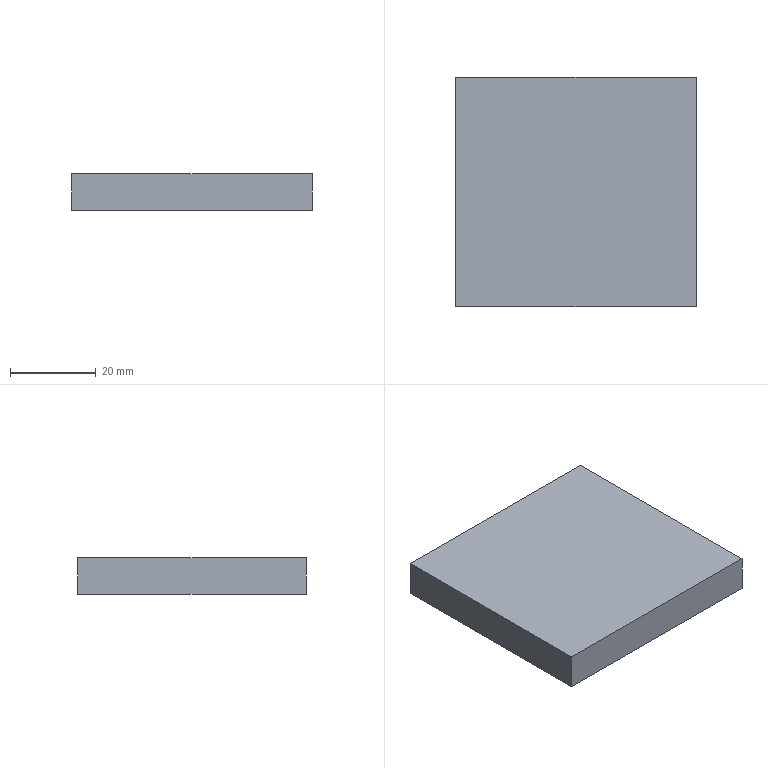NC program | NX | posted with a generic post | part box 56 x 53.3 x 8.5 mm
Lines 3580 to 5023 of 5023, first 1358 of 1432 lines:
(ZLEVEL_PROFILE_COPY_COPY , TOOL : D2)
N7134 T18 M6
N7136 G54
N7138 G17 G0 G90 X-10.995 Y-10.6 S9500 M3
N7140 G43 Z30. H18
N7142 Z-1.643
N7144 G94 G1 X-10.822 Y-10.9 F1000.
N7146 G3 X-10.648 Y-11. R0.2
N7148 G1 X-10. F1100.
N7150 G3 X-9.5 Y-10.5 R0.5
N7152 G1 Y-9.852
N7154 G3 X-9.6 Y-9.678 R0.2
N7156 G1 X-9.9 Y-9.505
N7158 G0 X-10.995 Y-10.6 Z-1.786
N7160 G1 X-10.822 Y-10.9 F1000.
N7162 G3 X-10.648 Y-11. R0.2
N7164 G1 X-10. F1100.
N7166 G3 X-9.5 Y-10.5 R0.5
N7168 G1 Y-9.852
N7170 G3 X-9.6 Y-9.678 R0.2
N7172 G1 X-9.9 Y-9.505
N7174 G0 X-10.995 Y-10.6 Z-1.929
N7176 G1 X-10.822 Y-10.9 F1000.
N7178 G3 X-10.648 Y-11. R0.2
N7180 G1 X-10. F1100.
N7182 G3 X-9.5 Y-10.5 R0.5
N7184 G1 Y-9.852
N7186 G3 X-9.6 Y-9.678 R0.2
N7188 G1 X-9.9 Y-9.505
N7190 G0 X-10.995 Y-10.6 Z-2.071
N7192 G1 X-10.822 Y-10.9 F1000.
N7194 G3 X-10.648 Y-11. R0.2
N7196 G1 X-10. F1100.
N7198 G3 X-9.5 Y-10.5 R0.5
N7200 G1 Y-9.852
N7202 G3 X-9.6 Y-9.678 R0.2
N7204 G1 X-9.9 Y-9.505
N7206 G0 X-10.995 Y-10.6 Z-2.214
N7208 G1 X-10.822 Y-10.9 F1000.
N7210 G3 X-10.648 Y-11. R0.2
N7212 G1 X-10. F1100.
N7214 G3 X-9.5 Y-10.5 R0.5
N7216 G1 Y-9.852
N7218 G3 X-9.6 Y-9.678 R0.2
N7220 G1 X-9.9 Y-9.505
N7222 G0 X-10.995 Y-10.6 Z-2.357
N7224 G1 X-10.822 Y-10.9 F1000.
N7226 G3 X-10.648 Y-11. R0.2
N7228 G1 X-10. F1100.
N7230 G3 X-9.5 Y-10.5 R0.5
N7232 G1 Y-9.852
N7234 G3 X-9.6 Y-9.678 R0.2
N7236 G1 X-9.9 Y-9.505
N7238 G0 X-10.995 Y-10.6 Z-2.5
N7240 G1 X-10.822 Y-10.9 F1000.
N7242 G3 X-10.648 Y-11. R0.2
N7244 G1 X-10. F1100.
N7246 G3 X-9.5 Y-10.5 R0.5
N7248 G1 Y-9.852
N7250 G3 X-9.6 Y-9.678 R0.2
N7252 G1 X-9.9 Y-9.505
N7254 G0 Z30.
N7256 X9.9
N7258 Z-1.643
N7260 G1 X9.6 Y-9.678 F1000.
N7262 G3 X9.5 Y-9.852 R0.2
N7264 G1 Y-10.5 F1100.
N7266 G3 X10. Y-11. R0.5
N7268 G1 X10.648
N7270 G3 X10.822 Y-10.9 R0.2
N7272 G1 X10.995 Y-10.6
N7274 G0 X9.9 Y-9.505 Z-1.786
N7276 G1 X9.6 Y-9.678 F1000.
N7278 G3 X9.5 Y-9.852 R0.2
N7280 G1 Y-10.5 F1100.
N7282 G3 X10. Y-11. R0.5
N7284 G1 X10.648
N7286 G3 X10.822 Y-10.9 R0.2
N7288 G1 X10.995 Y-10.6
N7290 G0 X9.9 Y-9.505 Z-1.929
N7292 G1 X9.6 Y-9.678 F1000.
N7294 G3 X9.5 Y-9.852 R0.2
N7296 G1 Y-10.5 F1100.
N7298 G3 X10. Y-11. R0.5
N7300 G1 X10.648
N7302 G3 X10.822 Y-10.9 R0.2
N7304 G1 X10.995 Y-10.6
N7306 G0 X9.9 Y-9.505 Z-2.071
N7308 G1 X9.6 Y-9.678 F1000.
N7310 G3 X9.5 Y-9.852 R0.2
N7312 G1 Y-10.5 F1100.
N7314 G3 X10. Y-11. R0.5
N7316 G1 X10.648
N7318 G3 X10.822 Y-10.9 R0.2
N7320 G1 X10.995 Y-10.6
N7322 G0 X9.9 Y-9.505 Z-2.214
N7324 G1 X9.6 Y-9.678 F1000.
N7326 G3 X9.5 Y-9.852 R0.2
N7328 G1 Y-10.5 F1100.
N7330 G3 X10. Y-11. R0.5
N7332 G1 X10.648
N7334 G3 X10.822 Y-10.9 R0.2
N7336 G1 X10.995 Y-10.6
N7338 G0 X9.9 Y-9.505 Z-2.357
N7340 G1 X9.6 Y-9.678 F1000.
N7342 G3 X9.5 Y-9.852 R0.2
N7344 G1 Y-10.5 F1100.
N7346 G3 X10. Y-11. R0.5
N7348 G1 X10.648
N7350 G3 X10.822 Y-10.9 R0.2
N7352 G1 X10.995 Y-10.6
N7354 G0 X9.9 Y-9.505 Z-2.5
N7356 G1 X9.6 Y-9.678 F1000.
N7358 G3 X9.5 Y-9.852 R0.2
N7360 G1 Y-10.5 F1100.
N7362 G3 X10. Y-11. R0.5
N7364 G1 X10.648
N7366 G3 X10.822 Y-10.9 R0.2
N7368 G1 X10.995 Y-10.6
N7370 G0 Z30.
N7372 X-20.908 Y-9.703
N7374 Z-1.643
N7376 G1 X-20.707 Y-9.425 F1000.
N7378 G3 X-20.686 Y-9.226 R0.2
N7380 G2 X-20.995 Y-8.5 R22.65 F1100.
N7382 G1 X-21.383
N7384 G2 X-21.769 Y-8.45 R1.5
N7386 G3 X-21.962 Y-8.502 R0.2
N7388 G1 X-22.183 Y-8.724
N7390 G0 X-20.908 Y-9.703 Z-1.786
N7392 G1 X-20.707 Y-9.425 F1000.
N7394 G3 X-20.686 Y-9.226 R0.2
N7396 G2 X-20.995 Y-8.5 R22.65 F1100.
N7398 G1 X-21.383
N7400 G2 X-21.769 Y-8.45 R1.5
N7402 G3 X-21.962 Y-8.502 R0.2
N7404 G1 X-22.183 Y-8.724
N7406 G0 X-20.908 Y-9.703 Z-1.929
N7408 G1 X-20.707 Y-9.425 F1000.
N7410 G3 X-20.686 Y-9.226 R0.2
N7412 G2 X-20.995 Y-8.5 R22.65 F1100.
N7414 G1 X-21.383
N7416 G2 X-21.769 Y-8.45 R1.5
N7418 G3 X-21.962 Y-8.502 R0.2
N7420 G1 X-22.183 Y-8.724
N7422 G0 X-20.908 Y-9.703 Z-2.071
N7424 G1 X-20.707 Y-9.425 F1000.
N7426 G3 X-20.686 Y-9.226 R0.2
N7428 G2 X-20.995 Y-8.5 R22.65 F1100.
N7430 G1 X-21.383
N7432 G2 X-21.769 Y-8.45 R1.5
N7434 G3 X-21.962 Y-8.502 R0.2
N7436 G1 X-22.183 Y-8.724
N7438 G0 X-20.908 Y-9.703 Z-2.214
N7440 G1 X-20.707 Y-9.425 F1000.
N7442 G3 X-20.686 Y-9.226 R0.2
N7444 G2 X-20.995 Y-8.5 R22.65 F1100.
N7446 G1 X-21.383
N7448 G2 X-21.769 Y-8.45 R1.5
N7450 G3 X-21.962 Y-8.502 R0.2
N7452 G1 X-22.183 Y-8.724
N7454 G0 X-20.908 Y-9.703 Z-2.357
N7456 G1 X-20.707 Y-9.425 F1000.
N7458 G3 X-20.686 Y-9.226 R0.2
N7460 G2 X-20.995 Y-8.5 R22.65 F1100.
N7462 G1 X-21.383
N7464 G2 X-21.769 Y-8.45 R1.5
N7466 G3 X-21.962 Y-8.502 R0.2
N7468 G1 X-22.183 Y-8.724
N7470 G0 X-20.908 Y-9.703 Z-2.5
N7472 G1 X-20.707 Y-9.425 F1000.
N7474 G3 X-20.686 Y-9.226 R0.2
N7476 G2 X-20.995 Y-8.5 R22.65 F1100.
N7478 G1 X-21.383
N7480 G2 X-21.769 Y-8.45 R1.5
N7482 G3 X-21.962 Y-8.502 R0.2
N7484 G1 X-22.183 Y-8.724
N7486 G0 X-20.908 Y-9.703 Z-2.65
N7488 G1 X-20.707 Y-9.425 F1000.
N7490 G3 X-20.686 Y-9.226 R0.2
N7492 G2 X-20.995 Y-8.5 R22.65 F1100.
N7494 G1 X-21.383
N7496 G2 X-21.769 Y-8.45 R1.5
N7498 G3 X-21.962 Y-8.502 R0.2
N7500 G1 X-22.183 Y-8.724
N7502 G0 X-20.908 Y-9.703 Z-2.8
N7504 G1 X-20.707 Y-9.425 F1000.
N7506 G3 X-20.686 Y-9.226 R0.2
N7508 G2 X-20.995 Y-8.5 R22.65 F1100.
N7510 G1 X-21.383
N7512 G2 X-21.769 Y-8.45 R1.5
N7514 G3 X-21.962 Y-8.502 R0.2
N7516 G1 X-22.183 Y-8.724
N7518 G0 X-20.908 Y-9.703 Z-2.95
N7520 G1 X-20.707 Y-9.425 F1000.
N7522 G3 X-20.686 Y-9.226 R0.2
N7524 G2 X-20.995 Y-8.5 R22.65 F1100.
N7526 G1 X-21.383
N7528 G2 X-21.769 Y-8.45 R1.5
N7530 G3 X-21.962 Y-8.502 R0.2
N7532 G1 X-22.183 Y-8.724
N7534 G0 X-20.908 Y-9.703 Z-3.1
N7536 G1 X-20.707 Y-9.425 F1000.
N7538 G3 X-20.686 Y-9.226 R0.2
N7540 G2 X-20.995 Y-8.5 R22.65 F1100.
N7542 G1 X-21.383
N7544 G2 X-21.769 Y-8.45 R1.5
N7546 G3 X-21.962 Y-8.502 R0.2
N7548 G1 X-22.183 Y-8.724
N7550 G0 X-20.908 Y-9.703 Z-3.233
N7552 G1 X-20.707 Y-9.425 F1000.
N7554 G3 X-20.686 Y-9.226 R0.2
N7556 G2 X-20.995 Y-8.5 R22.65 F1100.
N7558 G1 X-21.383
N7560 G2 X-21.769 Y-8.45 R1.5
N7562 G3 X-21.962 Y-8.502 R0.2
N7564 G1 X-22.183 Y-8.724
N7566 G0 X-20.908 Y-9.703 Z-3.367
N7568 G1 X-20.707 Y-9.425 F1000.
N7570 G3 X-20.686 Y-9.226 R0.2
N7572 G2 X-20.995 Y-8.5 R22.65 F1100.
N7574 G1 X-21.383
N7576 G2 X-21.769 Y-8.45 R1.5
N7578 G3 X-21.962 Y-8.502 R0.2
N7580 G1 X-22.183 Y-8.724
N7582 G0 X-20.908 Y-9.703 Z-3.5
N7584 G1 X-20.707 Y-9.425 F1000.
N7586 G3 X-20.686 Y-9.226 R0.2
N7588 G2 X-20.995 Y-8.5 R22.65 F1100.
N7590 G1 X-21.383
N7592 G2 X-21.769 Y-8.45 R1.5
N7594 G3 X-21.962 Y-8.502 R0.2
N7596 G1 X-22.183 Y-8.724
N7598 G0 Z30.
N7600 X-22.18 Y8.725
N7602 Z-1.643
N7604 G1 X-21.959 Y8.503 F1000.
N7606 G3 X-21.766 Y8.45 R0.2
N7608 G2 X-21.383 Y8.5 R1.5 F1100.
N7610 G1 X-20.995
N7612 G2 X-20.689 Y9.219 R22.65
N7614 G3 X-20.71 Y9.418 R0.2
N7616 G1 X-20.911 Y9.696
N7618 G0 X-22.18 Y8.725 Z-1.786
N7620 G1 X-21.959 Y8.503 F1000.
N7622 G3 X-21.766 Y8.45 R0.2
N7624 G2 X-21.383 Y8.5 R1.5 F1100.
N7626 G1 X-20.995
N7628 G2 X-20.689 Y9.22 R22.65
N7630 G3 X-20.709 Y9.419 R0.2
N7632 G1 X-20.911 Y9.697
N7634 G0 X-22.18 Y8.725 Z-1.929
N7636 G1 X-21.959 Y8.503 F1000.
N7638 G3 X-21.766 Y8.45 R0.2
N7640 G2 X-21.383 Y8.5 R1.5 F1100.
N7642 G1 X-20.995
N7644 G2 X-20.688 Y9.22 R22.65
N7646 G3 X-20.709 Y9.419 R0.2
N7648 G1 X-20.911 Y9.697
N7650 G0 X-22.18 Y8.725 Z-2.071
N7652 G1 X-21.96 Y8.503 F1000.
N7654 G3 X-21.767 Y8.45 R0.2
N7656 G2 X-21.383 Y8.5 R1.5 F1100.
N7658 G1 X-20.995
N7660 G2 X-20.688 Y9.221 R22.65
N7662 G3 X-20.709 Y9.42 R0.2
N7664 G1 X-20.911 Y9.698
N7666 G0 X-22.181 Y8.725 Z-2.214
N7668 G1 X-21.96 Y8.503 F1000.
N7670 G3 X-21.767 Y8.45 R0.2
N7672 G2 X-21.383 Y8.5 R1.5 F1100.
N7674 G1 X-20.995
N7676 G2 X-20.688 Y9.222 R22.65
N7678 G3 X-20.709 Y9.42 R0.2
N7680 G1 X-20.91 Y9.698
N7682 G0 X-22.181 Y8.725 Z-2.357
N7684 G1 X-21.96 Y8.502 F1000.
N7686 G3 X-21.767 Y8.45 R0.2
N7688 G2 X-21.383 Y8.5 R1.5 F1100.
N7690 G1 X-20.995
N7692 G2 X-20.688 Y9.222 R22.65
N7694 G3 X-20.708 Y9.421 R0.2
N7696 G1 X-20.91 Y9.699
N7698 G0 X-22.181 Y8.724 Z-2.5
N7700 G1 X-21.96 Y8.502 F1000.
N7702 G3 X-21.767 Y8.45 R0.2
N7704 G2 X-21.383 Y8.5 R1.5 F1100.
N7706 G1 X-20.995
N7708 G2 X-20.687 Y9.223 R22.65
N7710 G3 X-20.708 Y9.422 R0.2
N7712 G1 X-20.91 Y9.7
N7714 G0 X-22.181 Y8.724 Z-2.65
N7716 G1 X-21.961 Y8.502 F1000.
N7718 G3 X-21.768 Y8.45 R0.2
N7720 G2 X-21.383 Y8.5 R1.5 F1100.
N7722 G1 X-20.995
N7724 G2 X-20.687 Y9.223 R22.65
N7726 G3 X-20.708 Y9.422 R0.2
N7728 G1 X-20.91 Y9.7
N7730 G0 X-22.182 Y8.724 Z-2.8
N7732 G1 X-21.961 Y8.502 F1000.
N7734 G3 X-21.768 Y8.45 R0.2
N7736 G2 X-21.383 Y8.5 R1.5 F1100.
N7738 G1 X-20.995
N7740 G2 X-20.687 Y9.224 R22.65
N7742 G3 X-20.708 Y9.423 R0.2
N7744 G1 X-20.909 Y9.701
N7746 G0 X-22.182 Y8.724 Z-2.95
N7748 G1 X-21.961 Y8.502 F1000.
N7750 G3 X-21.768 Y8.45 R0.2
N7752 G2 X-21.383 Y8.5 R1.5 F1100.
N7754 G1 X-20.995
N7756 G2 X-20.686 Y9.225 R22.65
N7758 G3 X-20.707 Y9.423 R0.2
N7760 G1 X-20.909 Y9.701
N7762 G0 X-22.182 Y8.724 Z-3.1
N7764 G1 X-21.961 Y8.502 F1000.
N7766 G3 X-21.768 Y8.45 R0.2
N7768 G2 X-21.383 Y8.5 R1.5 F1100.
N7770 G1 X-20.995
N7772 G2 X-20.686 Y9.225 R22.65
N7774 G3 X-20.707 Y9.424 R0.2
N7776 G1 X-20.909 Y9.702
N7778 G0 X-22.183 Y8.724 Z-3.233
N7780 G1 X-21.962 Y8.502 F1000.
N7782 G3 X-21.769 Y8.45 R0.2
N7784 G2 X-21.383 Y8.5 R1.5 F1100.
N7786 G1 X-20.995
N7788 G2 X-20.686 Y9.226 R22.65
N7790 G3 X-20.707 Y9.425 R0.2
N7792 G1 X-20.908 Y9.703
N7794 G0 X-22.183 Y8.724 Z-3.367
N7796 G1 X-21.962 Y8.502 F1000.
N7798 G3 X-21.769 Y8.45 R0.2
N7800 G2 X-21.383 Y8.5 R1.5 F1100.
N7802 G1 X-20.995
N7804 G2 X-20.686 Y9.226 R22.65
N7806 G3 X-20.707 Y9.425 R0.2
N7808 G1 X-20.908 Y9.703
N7810 G0 X-22.183 Y8.724 Z-3.5
N7812 G1 X-21.962 Y8.502 F1000.
N7814 G3 X-21.769 Y8.45 R0.2
N7816 G2 X-21.383 Y8.5 R1.5 F1100.
N7818 G1 X-20.995
N7820 G2 X-20.686 Y9.227 R22.65
N7822 G3 X-20.706 Y9.426 R0.2
N7824 G1 X-20.908 Y9.704
N7826 G0 Z30.
N7828 X20.908 Y9.703
N7830 Z-1.643
N7832 G1 X20.707 Y9.425 F1000.
N7834 G3 X20.686 Y9.226 R0.2
N7836 G2 X20.995 Y8.5 R22.65 F1100.
N7838 G1 X21.383
N7840 G2 X21.769 Y8.45 R1.5
N7842 G3 X21.962 Y8.502 R0.2
N7844 G1 X22.183 Y8.724
N7846 G0 X20.908 Y9.703 Z-1.786
N7848 G1 X20.707 Y9.425 F1000.
N7850 G3 X20.686 Y9.226 R0.2
N7852 G2 X20.995 Y8.5 R22.65 F1100.
N7854 G1 X21.383
N7856 G2 X21.769 Y8.45 R1.5
N7858 G3 X21.962 Y8.502 R0.2
N7860 G1 X22.183 Y8.724
N7862 G0 X20.908 Y9.703 Z-1.929
N7864 G1 X20.707 Y9.425 F1000.
N7866 G3 X20.686 Y9.226 R0.2
N7868 G2 X20.995 Y8.5 R22.65 F1100.
N7870 G1 X21.383
N7872 G2 X21.769 Y8.45 R1.5
N7874 G3 X21.962 Y8.502 R0.2
N7876 G1 X22.183 Y8.724
N7878 G0 X20.908 Y9.703 Z-2.071
N7880 G1 X20.707 Y9.425 F1000.
N7882 G3 X20.686 Y9.226 R0.2
N7884 G2 X20.995 Y8.5 R22.65 F1100.
N7886 G1 X21.383
N7888 G2 X21.769 Y8.45 R1.5
N7890 G3 X21.962 Y8.502 R0.2
N7892 G1 X22.183 Y8.724
N7894 G0 X20.908 Y9.703 Z-2.214
N7896 G1 X20.707 Y9.425 F1000.
N7898 G3 X20.686 Y9.226 R0.2
N7900 G2 X20.995 Y8.5 R22.65 F1100.
N7902 G1 X21.383
N7904 G2 X21.769 Y8.45 R1.5
N7906 G3 X21.962 Y8.502 R0.2
N7908 G1 X22.183 Y8.724
N7910 G0 X20.908 Y9.703 Z-2.357
N7912 G1 X20.707 Y9.425 F1000.
N7914 G3 X20.686 Y9.226 R0.2
N7916 G2 X20.995 Y8.5 R22.65 F1100.
N7918 G1 X21.383
N7920 G2 X21.769 Y8.45 R1.5
N7922 G3 X21.962 Y8.502 R0.2
N7924 G1 X22.183 Y8.724
N7926 G0 X20.908 Y9.703 Z-2.5
N7928 G1 X20.707 Y9.425 F1000.
N7930 G3 X20.686 Y9.226 R0.2
N7932 G2 X20.995 Y8.5 R22.65 F1100.
N7934 G1 X21.383
N7936 G2 X21.769 Y8.45 R1.5
N7938 G3 X21.962 Y8.502 R0.2
N7940 G1 X22.183 Y8.724
N7942 G0 X20.908 Y9.703 Z-2.65
N7944 G1 X20.707 Y9.425 F1000.
N7946 G3 X20.686 Y9.226 R0.2
N7948 G2 X20.995 Y8.5 R22.65 F1100.
N7950 G1 X21.383
N7952 G2 X21.769 Y8.45 R1.5
N7954 G3 X21.962 Y8.502 R0.2
N7956 G1 X22.183 Y8.724
N7958 G0 X20.908 Y9.703 Z-2.8
N7960 G1 X20.707 Y9.425 F1000.
N7962 G3 X20.686 Y9.226 R0.2
N7964 G2 X20.995 Y8.5 R22.65 F1100.
N7966 G1 X21.383
N7968 G2 X21.769 Y8.45 R1.5
N7970 G3 X21.962 Y8.502 R0.2
N7972 G1 X22.183 Y8.724
N7974 G0 X20.908 Y9.703 Z-2.95
N7976 G1 X20.707 Y9.425 F1000.
N7978 G3 X20.686 Y9.226 R0.2
N7980 G2 X20.995 Y8.5 R22.65 F1100.
N7982 G1 X21.383
N7984 G2 X21.769 Y8.45 R1.5
N7986 G3 X21.962 Y8.502 R0.2
N7988 G1 X22.183 Y8.724
N7990 G0 X20.908 Y9.703 Z-3.1
N7992 G1 X20.707 Y9.425 F1000.
N7994 G3 X20.686 Y9.226 R0.2
N7996 G2 X20.995 Y8.5 R22.65 F1100.
N7998 G1 X21.383
N8000 G2 X21.769 Y8.45 R1.5
N8002 G3 X21.962 Y8.502 R0.2
N8004 G1 X22.183 Y8.724
N8006 G0 X20.908 Y9.703 Z-3.233
N8008 G1 X20.707 Y9.425 F1000.
N8010 G3 X20.686 Y9.226 R0.2
N8012 G2 X20.995 Y8.5 R22.65 F1100.
N8014 G1 X21.383
N8016 G2 X21.769 Y8.45 R1.5
N8018 G3 X21.962 Y8.502 R0.2
N8020 G1 X22.183 Y8.724
N8022 G0 X20.908 Y9.703 Z-3.367
N8024 G1 X20.707 Y9.425 F1000.
N8026 G3 X20.686 Y9.226 R0.2
N8028 G2 X20.995 Y8.5 R22.65 F1100.
N8030 G1 X21.383
N8032 G2 X21.769 Y8.45 R1.5
N8034 G3 X21.962 Y8.502 R0.2
N8036 G1 X22.183 Y8.724
N8038 G0 X20.908 Y9.703 Z-3.5
N8040 G1 X20.707 Y9.425 F1000.
N8042 G3 X20.686 Y9.226 R0.2
N8044 G2 X20.995 Y8.5 R22.65 F1100.
N8046 G1 X21.383
N8048 G2 X21.769 Y8.45 R1.5
N8050 G3 X21.962 Y8.502 R0.2
N8052 G1 X22.183 Y8.724
N8054 G0 Z30.
N8056 Y-8.724
N8058 Z-1.643
N8060 G1 X21.962 Y-8.502 F1000.
N8062 G3 X21.769 Y-8.45 R0.2
N8064 G2 X21.383 Y-8.5 R1.5 F1100.
N8066 G1 X20.995
N8068 G2 X20.686 Y-9.226 R22.65
N8070 G3 X20.707 Y-9.425 R0.2
N8072 G1 X20.908 Y-9.703
N8074 G0 X22.183 Y-8.724 Z-1.786
N8076 G1 X21.962 Y-8.502 F1000.
N8078 G3 X21.769 Y-8.45 R0.2
N8080 G2 X21.383 Y-8.5 R1.5 F1100.
N8082 G1 X20.995
N8084 G2 X20.686 Y-9.226 R22.65
N8086 G3 X20.707 Y-9.425 R0.2
N8088 G1 X20.908 Y-9.703
N8090 G0 X22.183 Y-8.724 Z-1.929
N8092 G1 X21.962 Y-8.502 F1000.
N8094 G3 X21.769 Y-8.45 R0.2
N8096 G2 X21.383 Y-8.5 R1.5 F1100.
N8098 G1 X20.995
N8100 G2 X20.686 Y-9.226 R22.65
N8102 G3 X20.707 Y-9.425 R0.2
N8104 G1 X20.908 Y-9.703
N8106 G0 X22.183 Y-8.724 Z-2.071
N8108 G1 X21.962 Y-8.502 F1000.
N8110 G3 X21.769 Y-8.45 R0.2
N8112 G2 X21.383 Y-8.5 R1.5 F1100.
N8114 G1 X20.995
N8116 G2 X20.686 Y-9.226 R22.65
N8118 G3 X20.707 Y-9.425 R0.2
N8120 G1 X20.908 Y-9.703
N8122 G0 X22.183 Y-8.724 Z-2.214
N8124 G1 X21.962 Y-8.502 F1000.
N8126 G3 X21.769 Y-8.45 R0.2
N8128 G2 X21.383 Y-8.5 R1.5 F1100.
N8130 G1 X20.995
N8132 G2 X20.686 Y-9.226 R22.65
N8134 G3 X20.707 Y-9.425 R0.2
N8136 G1 X20.908 Y-9.703
N8138 G0 X22.183 Y-8.724 Z-2.357
N8140 G1 X21.962 Y-8.502 F1000.
N8142 G3 X21.769 Y-8.45 R0.2
N8144 G2 X21.383 Y-8.5 R1.5 F1100.
N8146 G1 X20.995
N8148 G2 X20.686 Y-9.226 R22.65
N8150 G3 X20.707 Y-9.425 R0.2
N8152 G1 X20.908 Y-9.703
N8154 G0 X22.183 Y-8.724 Z-2.5
N8156 G1 X21.962 Y-8.502 F1000.
N8158 G3 X21.769 Y-8.45 R0.2
N8160 G2 X21.383 Y-8.5 R1.5 F1100.
N8162 G1 X20.995
N8164 G2 X20.686 Y-9.226 R22.65
N8166 G3 X20.707 Y-9.425 R0.2
N8168 G1 X20.908 Y-9.703
N8170 G0 X22.183 Y-8.724 Z-2.65
N8172 G1 X21.962 Y-8.502 F1000.
N8174 G3 X21.769 Y-8.45 R0.2
N8176 G2 X21.383 Y-8.5 R1.5 F1100.
N8178 G1 X20.995
N8180 G2 X20.686 Y-9.226 R22.65
N8182 G3 X20.707 Y-9.425 R0.2
N8184 G1 X20.908 Y-9.703
N8186 G0 X22.183 Y-8.724 Z-2.8
N8188 G1 X21.962 Y-8.502 F1000.
N8190 G3 X21.769 Y-8.45 R0.2
N8192 G2 X21.383 Y-8.5 R1.5 F1100.
N8194 G1 X20.995
N8196 G2 X20.686 Y-9.226 R22.65
N8198 G3 X20.707 Y-9.425 R0.2
N8200 G1 X20.908 Y-9.703
N8202 G0 X22.183 Y-8.724 Z-2.95
N8204 G1 X21.962 Y-8.502 F1000.
N8206 G3 X21.769 Y-8.45 R0.2
N8208 G2 X21.383 Y-8.5 R1.5 F1100.
N8210 G1 X20.995
N8212 G2 X20.686 Y-9.226 R22.65
N8214 G3 X20.707 Y-9.425 R0.2
N8216 G1 X20.908 Y-9.703
N8218 G0 X22.183 Y-8.724 Z-3.1
N8220 G1 X21.962 Y-8.502 F1000.
N8222 G3 X21.769 Y-8.45 R0.2
N8224 G2 X21.383 Y-8.5 R1.5 F1100.
N8226 G1 X20.995
N8228 G2 X20.686 Y-9.226 R22.65
N8230 G3 X20.707 Y-9.425 R0.2
N8232 G1 X20.908 Y-9.703
N8234 G0 X22.183 Y-8.724 Z-3.233
N8236 G1 X21.962 Y-8.502 F1000.
N8238 G3 X21.769 Y-8.45 R0.2
N8240 G2 X21.383 Y-8.5 R1.5 F1100.
N8242 G1 X20.995
N8244 G2 X20.686 Y-9.226 R22.65
N8246 G3 X20.707 Y-9.425 R0.2
N8248 G1 X20.908 Y-9.703
N8250 G0 X22.183 Y-8.724 Z-3.367
N8252 G1 X21.962 Y-8.502 F1000.
N8254 G3 X21.769 Y-8.45 R0.2
N8256 G2 X21.383 Y-8.5 R1.5 F1100.
N8258 G1 X20.995
N8260 G2 X20.686 Y-9.226 R22.65
N8262 G3 X20.707 Y-9.425 R0.2
N8264 G1 X20.908 Y-9.703
N8266 G0 X22.183 Y-8.724 Z-3.5
N8268 G1 X21.962 Y-8.502 F1000.
N8270 G3 X21.769 Y-8.45 R0.2
N8272 G2 X21.383 Y-8.5 R1.5 F1100.
N8274 G1 X20.995
N8276 G2 X20.686 Y-9.226 R22.65
N8278 G3 X20.707 Y-9.425 R0.2
N8280 G1 X20.908 Y-9.703
N8282 G0 Z30.
N8284 X0.346 Y-17.4
N8286 Z-1.643
N8288 G1 X0.173 Y-17.1 F1000.
N8290 G3 X0. Y-17. R0.2
N8292 G1 X-7.776 F1100.
N8294 G3 X-7.979 Y-17.957 R0.5
N8296 X7.979 Y-17.957 R19.65
N8298 X7.776 Y-17. R0.5
N8300 G1 X0.
N8302 G3 X-0.173 Y-17.1 R0.2
N8304 G1 X-0.346 Y-17.4
N8306 G0 X0.346 Z-1.786
N8308 G1 X0.173 Y-17.1 F1000.
N8310 G3 X0. Y-17. R0.2
N8312 G1 X-7.776 F1100.
N8314 G3 X-7.979 Y-17.957 R0.5
N8316 X7.979 Y-17.957 R19.65
N8318 X7.776 Y-17. R0.5
N8320 G1 X0.
N8322 G3 X-0.173 Y-17.1 R0.2
N8324 G1 X-0.346 Y-17.4
N8326 G0 X0.346 Z-1.929
N8328 G1 X0.173 Y-17.1 F1000.
N8330 G3 X0. Y-17. R0.2
N8332 G1 X-7.776 F1100.
N8334 G3 X-7.979 Y-17.957 R0.5
N8336 X7.979 Y-17.957 R19.65
N8338 X7.776 Y-17. R0.5
N8340 G1 X0.
N8342 G3 X-0.173 Y-17.1 R0.2
N8344 G1 X-0.346 Y-17.4
N8346 G0 X0.346 Z-2.071
N8348 G1 X0.173 Y-17.1 F1000.
N8350 G3 X0. Y-17. R0.2
N8352 G1 X-7.776 F1100.
N8354 G3 X-7.979 Y-17.957 R0.5
N8356 X7.979 Y-17.957 R19.65
N8358 X7.776 Y-17. R0.5
N8360 G1 X0.
N8362 G3 X-0.173 Y-17.1 R0.2
N8364 G1 X-0.346 Y-17.4
N8366 G0 X0.346 Z-2.214
N8368 G1 X0.173 Y-17.1 F1000.
N8370 G3 X0. Y-17. R0.2
N8372 G1 X-7.776 F1100.
N8374 G3 X-7.979 Y-17.957 R0.5
N8376 X7.979 Y-17.957 R19.65
N8378 X7.776 Y-17. R0.5
N8380 G1 X0.
N8382 G3 X-0.173 Y-17.1 R0.2
N8384 G1 X-0.346 Y-17.4
N8386 G0 X0.346 Z-2.357
N8388 G1 X0.173 Y-17.1 F1000.
N8390 G3 X0. Y-17. R0.2
N8392 G1 X-7.776 F1100.
N8394 G3 X-7.979 Y-17.957 R0.5
N8396 X7.979 Y-17.957 R19.65
N8398 X7.776 Y-17. R0.5
N8400 G1 X0.
N8402 G3 X-0.173 Y-17.1 R0.2
N8404 G1 X-0.346 Y-17.4
N8406 G0 X0.346 Z-2.5
N8408 G1 X0.173 Y-17.1 F1000.
N8410 G3 X0. Y-17. R0.2
N8412 G1 X-7.776 F1100.
N8414 G3 X-7.979 Y-17.957 R0.5
N8416 X7.979 Y-17.957 R19.65
N8418 X7.776 Y-17. R0.5
N8420 G1 X0.
N8422 G3 X-0.173 Y-17.1 R0.2
N8424 G1 X-0.346 Y-17.4
N8426 G0 Z30.
N8428 X16.4 Y0.995
N8430 Z-2.65
N8432 G1 X16.1 Y0.822 F1000.
N8434 G3 X16. Y0.648 R0.2
N8436 G1 Y-0.173 F1100.
N8438 X15.998 Y-0.499
N8440 X16.002 Y-0.503
N8442 X16.059 Y-0.5
N8444 X17.148
N8446 G3 X17.322 Y-0.4 R0.2
N8448 G1 X17.495 Y-0.1
N8450 G0 X16.4 Y0.995 Z-2.8
N8452 G1 X16.1 Y0.822 F1000.
N8454 G3 X16. Y0.648 R0.2
N8456 G1 Y-0.173 F1100.
N8458 X15.999 Y-0.498
N8460 X16.002 Y-0.5
N8462 X17.148
N8464 G3 X17.322 Y-0.4 R0.2
N8466 G1 X17.495 Y-0.1
N8468 G0 X16.4 Y0.995 Z-2.95
N8470 G1 X16.1 Y0.822 F1000.
N8472 G3 X16. Y0.648 R0.2
N8474 G1 Y-0.5 F1100.
N8476 X17.148
N8478 G3 X17.322 Y-0.4 R0.2
N8480 G1 X17.495 Y-0.1
N8482 G0 X16.4 Y0.995 Z-3.1
N8484 G1 X16.1 Y0.822 F1000.
N8486 G3 X16. Y0.648 R0.2
N8488 G1 Y-0.499 F1100.
N8490 X16.059 Y-0.5
N8492 X17.148
N8494 G3 X17.322 Y-0.4 R0.2
N8496 G1 X17.495 Y-0.1
N8498 G0 Z30.
N8500 X18.505
N8502 Z-2.65
N8504 G1 X18.678 Y-0.4 F1000.
N8506 G3 X18.852 Y-0.5 R0.2
N8508 G1 X20. F1100.
N8510 Y0.648
N8512 G3 X19.9 Y0.822 R0.2
N8514 G1 X19.6 Y0.995
N8516 G0 X18.505 Y-0.1 Z-2.8
N8518 G1 X18.678 Y-0.4 F1000.
N8520 G3 X18.852 Y-0.5 R0.2
N8522 G1 X20. F1100.
N8524 Y0.648
N8526 G3 X19.9 Y0.822 R0.2
N8528 G1 X19.6 Y0.995
N8530 G0 X18.505 Y-0.1 Z-2.95
N8532 G1 X18.678 Y-0.4 F1000.
N8534 G3 X18.852 Y-0.5 R0.2
N8536 G1 X20. F1100.
N8538 Y0.648
N8540 G3 X19.9 Y0.822 R0.2
N8542 G1 X19.6 Y0.995
N8544 G0 X18.505 Y-0.1 Z-3.1
N8546 G1 X18.678 Y-0.4 F1000.
N8548 G3 X18.852 Y-0.5 R0.2
N8550 G1 X20. F1100.
N8552 Y0.648
N8554 G3 X19.9 Y0.822 R0.2
N8556 G1 X19.6 Y0.995
N8558 G0 Z30.
N8560 Y3.005
N8562 Z-2.65
N8564 G1 X19.9 Y3.178 F1000.
N8566 G3 X20. Y3.352 R0.2
N8568 G1 Y4.5 F1100.
N8570 X18.852
N8572 G3 X18.678 Y4.4 R0.2
N8574 G1 X18.505 Y4.1
N8576 G0 X19.6 Y3.005 Z-2.8
N8578 G1 X19.9 Y3.178 F1000.
N8580 G3 X20. Y3.352 R0.2
N8582 G1 Y4.5 F1100.
N8584 X18.852
N8586 G3 X18.678 Y4.4 R0.2
N8588 G1 X18.505 Y4.1
N8590 G0 X19.6 Y3.005 Z-2.95
N8592 G1 X19.9 Y3.178 F1000.
N8594 G3 X20. Y3.352 R0.2
N8596 G1 Y4.5 F1100.
N8598 X18.852
N8600 G3 X18.678 Y4.4 R0.2
N8602 G1 X18.505 Y4.1
N8604 G0 X19.6 Y3.005 Z-3.1
N8606 G1 X19.9 Y3.178 F1000.
N8608 G3 X20. Y3.352 R0.2
N8610 G1 Y4.5 F1100.
N8612 X18.852
N8614 G3 X18.678 Y4.4 R0.2
N8616 G1 X18.505 Y4.1
N8618 G0 Z30.
N8620 X17.495
N8622 Z-2.65
N8624 G1 X17.322 Y4.4 F1000.
N8626 G3 X17.148 Y4.5 R0.2
N8628 G1 X16.059 F1100.
N8630 X16.
N8632 Y3.352
N8634 G3 X16.1 Y3.178 R0.2
N8636 G1 X16.4 Y3.005
N8638 G0 X17.495 Y4.1 Z-2.8
N8640 G1 X17.322 Y4.4 F1000.
N8642 G3 X17.148 Y4.5 R0.2
N8644 G1 X16.059 F1100.
N8646 X16.
N8648 Y3.352
N8650 G3 X16.1 Y3.178 R0.2
N8652 G1 X16.4 Y3.005
N8654 G0 X17.495 Y4.1 Z-2.95
N8656 G1 X17.322 Y4.4 F1000.
N8658 G3 X17.148 Y4.5 R0.2
N8660 G1 X16. F1100.
N8662 Y3.352
N8664 G3 X16.1 Y3.178 R0.2
N8666 G1 X16.4 Y3.005
N8668 G0 X17.495 Y4.1 Z-3.1
N8670 G1 X17.322 Y4.4 F1000.
N8672 G3 X17.148 Y4.5 R0.2
N8674 G1 X16.059 F1100.
N8676 X16. Y4.499
N8678 Y3.352
N8680 G3 X16.1 Y3.178 R0.2
N8682 G1 X16.4 Y3.005
N8684 G0 Z30.
N8686 X-0.995 Y-0.6
N8688 Z-2.65
N8690 G1 X-0.822 Y-0.9 F1000.
N8692 G3 X-0.648 Y-1. R0.2
N8694 G1 X0.5 F1100.
N8696 Y0.148
N8698 G3 X0.4 Y0.322 R0.2
N8700 G1 X0.1 Y0.495
N8702 G0 X-0.995 Y-0.6 Z-2.8
N8704 G1 X-0.822 Y-0.9 F1000.
N8706 G3 X-0.648 Y-1. R0.2
N8708 G1 X0.5 F1100.
N8710 Y0.148
N8712 G3 X0.4 Y0.322 R0.2
N8714 G1 X0.1 Y0.495
N8716 G0 X-0.995 Y-0.6 Z-2.95
N8718 G1 X-0.822 Y-0.9 F1000.
N8720 G3 X-0.648 Y-1. R0.2
N8722 G1 X0.5 F1100.
N8724 Y0.148
N8726 G3 X0.4 Y0.322 R0.2
N8728 G1 X0.1 Y0.495
N8730 G0 X-0.995 Y-0.6 Z-3.1
N8732 G1 X-0.822 Y-0.9 F1000.
N8734 G3 X-0.648 Y-1. R0.2
N8736 G1 X0.5 F1100.
N8738 Y0.148
N8740 G3 X0.4 Y0.322 R0.2
N8742 G1 X0.1 Y0.495
N8744 G0 Z30.
N8746 Y5.005
N8748 Z-2.65
N8750 G1 X0.4 Y5.178 F1000.
N8752 G3 X0.5 Y5.352 R0.2
N8754 G1 Y6.5 F1100.
N8756 X-0.648
N8758 G3 X-0.822 Y6.4 R0.2
N8760 G1 X-0.995 Y6.1
N8762 G0 X0.1 Y5.005 Z-2.8
N8764 G1 X0.4 Y5.178 F1000.
N8766 G3 X0.5 Y5.352 R0.2
N8768 G1 Y6.5 F1100.
N8770 X-0.648
N8772 G3 X-0.822 Y6.4 R0.2
N8774 G1 X-0.995 Y6.1
N8776 G0 X0.1 Y5.005 Z-2.95
N8778 G1 X0.4 Y5.178 F1000.
N8780 G3 X0.5 Y5.352 R0.2
N8782 G1 Y6.5 F1100.
N8784 X-0.648
N8786 G3 X-0.822 Y6.4 R0.2
N8788 G1 X-0.995 Y6.1
N8790 G0 X0.1 Y5.005 Z-3.1
N8792 G1 X0.4 Y5.178 F1000.
N8794 G3 X0.5 Y5.352 R0.2
N8796 G1 Y6.5 F1100.
N8798 X-0.648
N8800 G3 X-0.822 Y6.4 R0.2
N8802 G1 X-0.995 Y6.1
N8804 G0 Z30.
N8806 X-6.005
N8808 Z-2.65
N8810 G1 X-6.178 Y6.4 F1000.
N8812 G3 X-6.352 Y6.5 R0.2
N8814 G1 X-7.425 F1100.
N8816 X-7.5
N8818 Y5.352
N8820 G3 X-7.4 Y5.178 R0.2
N8822 G1 X-7.1 Y5.005
N8824 G0 X-6.005 Y6.1 Z-2.8
N8826 G1 X-6.178 Y6.4 F1000.
N8828 G3 X-6.352 Y6.5 R0.2
N8830 G1 X-7.425 F1100.
N8832 X-7.5
N8834 Y5.352
N8836 G3 X-7.4 Y5.178 R0.2
N8838 G1 X-7.1 Y5.005
N8840 G0 X-6.005 Y6.1 Z-2.95
N8842 G1 X-6.178 Y6.4 F1000.
N8844 G3 X-6.352 Y6.5 R0.2
N8846 G1 X-7.5 F1100.
N8848 Y5.352
N8850 G3 X-7.4 Y5.178 R0.2
N8852 G1 X-7.1 Y5.005
N8854 G0 X-6.005 Y6.1 Z-3.1
N8856 G1 X-6.178 Y6.4 F1000.
N8858 G3 X-6.352 Y6.5 R0.2
N8860 G1 X-7.425 F1100.
N8862 X-7.5 Y6.499
N8864 Y5.352
N8866 G3 X-7.4 Y5.178 R0.2
N8868 G1 X-7.1 Y5.005
N8870 G0 Z30.
N8872 Y0.495
N8874 Z-2.65
N8876 G1 X-7.4 Y0.322 F1000.
N8878 G3 X-7.5 Y0.148 R0.2
N8880 G1 Y-1. F1100.
N8882 X-6.352
N8884 G3 X-6.178 Y-0.9 R0.2
N8886 G1 X-6.005 Y-0.6
N8888 G0 X-7.1 Y0.495 Z-2.8
N8890 G1 X-7.4 Y0.322 F1000.
N8892 G3 X-7.5 Y0.148 R0.2
N8894 G1 Y-1. F1100.
N8896 X-6.352
N8898 G3 X-6.178 Y-0.9 R0.2
N8900 G1 X-6.005 Y-0.6
N8902 G0 X-7.1 Y0.495 Z-2.95
N8904 G1 X-7.4 Y0.322 F1000.
N8906 G3 X-7.5 Y0.148 R0.2
N8908 G1 Y-1. F1100.
N8910 X-6.352
N8912 G3 X-6.178 Y-0.9 R0.2
N8914 G1 X-6.005 Y-0.6
N8916 G0 X-7.1 Y0.495 Z-3.1
N8918 G1 X-7.4 Y0.322 F1000.
N8920 G3 X-7.5 Y0.148 R0.2
N8922 G1 X-7.499 Y-1. F1100.
N8924 X-6.352
N8926 G3 X-6.178 Y-0.9 R0.2
N8928 G1 X-6.005 Y-0.6
N8930 G0 Z30.
N8932 M5
(PLANAR_MILL_COPY_COPY_COPY_COPY_COPY_COPY_1_COPY_1_COPY , TOOL : D6A45)
N8934 T01 M6
N8936 G54
N8938 G17 G0 G90 X-19.65 Y9.134 S9500 M3
N8940 G43 Z30. H1
N8942 Z0.5
N8944 G94 G1 Z-1. F1250.
N8946 G3 X-19.15 Y10. R1.
N8948 G2 X-16. Y13.15 R3.15
N8950 X-19.15 Y10. R-3.15
N8952 G3 X-19.65 Y10.866 R1.
N8954 G1 Z0.5
N8956 G0 Z30.
N8958 X-15.935 Y9.891
N8960 Z0.5
N8962 G1 Z-1.
N8964 G3 X-15.7 Y10. R0.5
N8966 X-16. Y10.3 R0.3
N8968 X-15.7 Y10. R-0.3
N8970 X-15.935 Y10.109 R0.5
N8972 G1 Z0.5
N8974 G0 Z30.
N8976 X12.35 Y-10.866
N8978 Z0.5
N8980 G1 Z-1.
N8982 G3 X12.85 Y-10. R1.
N8984 G2 X16. Y-6.85 R3.15
N8986 X12.85 Y-10. R-3.15
N8988 G3 X12.35 Y-9.134 R1.
N8990 G1 Z0.5
N8992 G0 Z30.
N8994 X16.065 Y-10.109
N8996 Z0.5
N8998 G1 Z-1.
N9000 G3 X16.3 Y-10. R0.5
N9002 X16. Y-9.7 R0.3
N9004 X16.3 Y-10. R-0.3
N9006 X16.065 Y-9.891 R0.5
N9008 G1 Z0.5
N9010 G0 Z30.
(PLANAR_MILL_COPY_COPY_COPY_COPY_COPY_COPY_1_COPY_1_COPY_COPY , TOOL : D6A45)
N9012 X1.27 Y-17.8
N9014 Z-0.7
N9016 G1 Z-2.2
N9018 X0.866 Y-17.1
N9020 G3 X0. Y-16.6 R1.
N9022 G1 X-7.776
N9024 G3 X-8.142 Y-18.322 R0.9
N9026 X8.142 Y-18.322 R20.05
N9028 X7.776 Y-16.6 R0.9
N9030 G1 X0.
N9032 G3 X-0.866 Y-17.1 R1.
N9034 G1 X-1.27 Y-17.8
N9036 Z-0.7
N9038 G0 Z30.
N9040 X14.403 Y-15.939
N9042 Z-0.7
N9044 G1 Z-2.2
N9046 X13.076 Y-14.68
N9048 G3 X12.751 Y-13.734 R1.
N9050 X12.859 Y-14.817 R1.45
N9052 G2 X11.753 Y-18.893 R3.1
N9054 X-11.753 Y-18.893 R22.25
N9056 X-12.859 Y-14.817 R3.1
N9058 G3 X-14.817 Y-12.859 R1.45
N9060 G2 X-18.893 Y-11.753 R3.1
N9062 X-20.624 Y-8.35 R22.25
N9064 G3 X-20.995 Y-8.1 R0.4
N9066 G1 X-21.383
N9068 G2 X-22.429 Y-7.342 R1.1
N9070 X-22.429 Y7.342 R23.6
N9072 X-21.383 Y8.1 R1.1
N9074 G1 X-20.995
N9076 G3 X-20.649 Y8.299 R0.4
N9078 X-21.416 Y8.941 R1.
N9080 G1 X-22.323 Y9.099
N9082 Z-0.7
N9084 G0 Z30.
N9086 X-14.403 Y15.939
N9088 Z-0.7
N9090 G1 Z-2.2
N9092 X-13.076 Y14.68
N9094 G3 X-12.751 Y13.734 R1.
N9096 X-12.859 Y14.817 R1.45
N9098 G2 X-11.753 Y18.893 R3.1
N9100 X11.753 Y18.893 R22.25
N9102 X12.859 Y14.817 R3.1
N9104 G3 X14.817 Y12.859 R1.45
N9106 G2 X18.893 Y11.753 R3.1
N9108 X20.624 Y8.35 R22.25
N9110 G3 X20.995 Y8.1 R0.4
N9112 G1 X21.383
N9114 G2 X22.429 Y7.342 R1.1
N9116 X22.429 Y-7.342 R23.6
N9118 X21.383 Y-8.1 R1.1
N9120 G1 X20.995
N9122 G3 X20.649 Y-8.299 R0.4
N9124 X21.416 Y-8.941 R1.
N9126 G1 X22.323 Y-9.099
N9128 Z-0.7
N9130 G0 Z30.
N9132 X19.329 Y-4.829
N9134 Z-0.7
N9136 G1 Z-2.2
N9138 X19.166 Y-5.48
N9140 G3 X19.441 Y-6.442 R1.
N9142 G2 X19.953 Y-6.149 R2.6
N9144 G3 X20.758 Y-5.203 R1.4
N9146 X20.758 Y5.203 R21.4
N9148 X19.953 Y6.149 R1.4
N9150 G2 X18.571 Y7.557 R2.6
N9152 G3 X17.271 Y10.184 R20.05
N9154 X15.532 Y10.767 R1.4
N9156 G2 X10.767 Y15.532 R3.65
N9158 G3 X10.184 Y17.271 R1.4
N9160 X-10.184 Y17.271 R20.05
N9162 X-10.767 Y15.532 R1.4
N9164 G2 X-11.374 Y11.763 R3.65
N9166 G3 X-10.599 Y11.131 R1.
N9168 G1 X-9.936 Y11.025
N9170 Z-0.7
N9172 G0 Z30.
N9174 X-19.329 Y4.829
N9176 Z-0.7
N9178 G1 Z-2.2
N9180 X-19.166 Y5.48
N9182 G3 X-19.441 Y6.442 R1.
N9184 G2 X-19.953 Y6.149 R2.6
N9186 G3 X-20.758 Y5.203 R1.4
N9188 X-20.758 Y-5.203 R21.4
N9190 X-19.953 Y-6.149 R1.4
N9192 G2 X-18.571 Y-7.557 R2.6
N9194 G3 X-17.271 Y-10.184 R20.05
N9196 X-15.532 Y-10.767 R1.4
N9198 G2 X-11.954 Y-11.22 R3.65
N9200 G3 X-11.415 Y-11.4 R0.9
N9202 G1 X-10.
N9204 G3 X-9.1 Y-10.5 R0.9
N9206 G1 Y-5.5
N9208 G2 X-7. Y-3.4 R2.1
N9210 G1 X7.
N9212 G2 X9.1 Y-5.5 R2.1
N9214 G1 Y-10.5
N9216 G3 X10. Y-11.4 R0.9
N9218 G1 X11.252
N9220 G3 X10.528 Y-10.711 R1.
N9222 G1 X10.3 Y-7.691
N9224 Z-0.7
N9226 G0 Z30.
N9228 M5
(HOLE_MILLING_1 , TOOL : D1.5)
N9230 T20 M6
N9232 G54
N9234 G17 G0 G90 X-4.1 Y18.5 S9500 M3
N9236 G43 Z30. H20
N9238 Z-2.
N9240 G94 G3 X-4.225 Y18.625 R0.125 F850.
N9242 X-4.35 Y18.5 R0.125
N9244 X-4.35 Y18.5 Z-2.08 I0.25 J0.
N9246 X-4.35 Y18.5 Z-2.16 I0.25 J0.
N9248 X-4.35 Y18.5 Z-2.24 I0.25 J0.
N9250 X-4.35 Y18.5 Z-2.32 I0.25 J0.
N9252 X-4.35 Y18.5 Z-2.4 I0.25 J0.
N9254 X-4.35 Y18.5 Z-2.48 I0.25 J0.
N9256 X-4.35 Y18.5 Z-2.56 I0.25 J0.
N9258 X-4.35 Y18.5 Z-2.64 I0.25 J0.
N9260 X-4.35 Y18.5 Z-2.72 I0.25 J0.
N9262 X-4.35 Y18.5 Z-2.8 I0.25 J0.
N9264 X-4.35 Y18.5 Z-2.88 I0.25 J0.
N9266 X-4.35 Y18.5 Z-2.96 I0.25 J0.
N9268 X-4.35 Y18.5 Z-3.04 I0.25 J0.
N9270 X-4.35 Y18.5 Z-3.12 I0.25 J0.
N9272 X-4.35 Y18.5 Z-3.2 I0.25 J0.
N9274 X-4.35 Y18.5 Z-3.28 I0.25 J0.
N9276 X-4.35 Y18.5 Z-3.36 I0.25 J0.
N9278 X-4.35 Y18.5 Z-3.44 I0.25 J0.
N9280 X-4.1 Y18.75 Z-3.5 R-0.25
N9282 X-4.35 Y18.5 R0.25
N9284 X-4.1 Y18.75 R-0.25
N9286 X-4.225 Y18.625 R0.125
N9288 X-4.1 Y18.5 R0.125
N9290 G0 Z30.
N9292 X10.4 Y16.2
N9294 Z-2.
N9296 G3 X10.275 Y16.325 R0.125
N9298 X10.15 Y16.2 R0.125
N9300 X10.15 Y16.2 Z-2.08 I0.25 J0.
N9302 X10.15 Y16.2 Z-2.16 I0.25 J0.
N9304 X10.15 Y16.2 Z-2.24 I0.25 J0.
N9306 X10.15 Y16.2 Z-2.32 I0.25 J0.
N9308 X10.15 Y16.2 Z-2.4 I0.25 J0.
N9310 X10.15 Y16.2 Z-2.48 I0.25 J0.
N9312 X10.15 Y16.2 Z-2.56 I0.25 J0.
N9314 X10.15 Y16.2 Z-2.64 I0.25 J0.
N9316 X10.15 Y16.2 Z-2.72 I0.25 J0.
N9318 X10.15 Y16.2 Z-2.8 I0.25 J0.
N9320 X10.15 Y16.2 Z-2.88 I0.25 J0.
N9322 X10.15 Y16.2 Z-2.96 I0.25 J0.
N9324 X10.15 Y16.2 Z-3.04 I0.25 J0.
N9326 X10.15 Y16.2 Z-3.12 I0.25 J0.
N9328 X10.15 Y16.2 Z-3.2 I0.25 J0.
N9330 X10.15 Y16.2 Z-3.28 I0.25 J0.
N9332 X10.15 Y16.2 Z-3.36 I0.25 J0.
N9334 X10.15 Y16.2 Z-3.44 I0.25 J0.
N9336 X10.4 Y16.45 Z-3.5 R-0.25
N9338 X10.15 Y16.2 R0.25
N9340 X10.4 Y16.45 R-0.25
N9342 X10.275 Y16.325 R0.125
N9344 X10.4 Y16.2 R0.125
N9346 G0 Z30.
(HOLE_MILLING_1_COPY , TOOL : D1.5)
N9348 X16. Y-10.
N9350 Z0.5
N9352 G3 X15.775 Y-9.775 R0.225
N9354 X15.55 Y-10. R0.225
N9356 X15.55 Y-10. Z0.42 I0.45 J0.
N9358 X15.55 Y-10. Z0.34 I0.45 J0.
N9360 X15.55 Y-10. Z0.26 I0.45 J0.
N9362 X15.55 Y-10. Z0.18 I0.45 J0.
N9364 X15.55 Y-10. Z0.1 I0.45 J0.
N9366 X15.55 Y-10. Z0.02 I0.45 J0.
N9368 X15.55 Y-10. Z-0.06 I0.45 J0.
N9370 X15.55 Y-10. Z-0.14 I0.45 J0.
N9372 X15.55 Y-10. Z-0.22 I0.45 J0.
N9374 X15.55 Y-10. Z-0.3 I0.45 J0.
N9376 X15.55 Y-10. Z-0.38 I0.45 J0.
N9378 X15.55 Y-10. Z-0.46 I0.45 J0.
N9380 X15.55 Y-10. Z-0.54 I0.45 J0.
N9382 X15.55 Y-10. Z-0.62 I0.45 J0.
N9384 X15.55 Y-10. Z-0.7 I0.45 J0.
N9386 X15.55 Y-10. Z-0.78 I0.45 J0.
N9388 X15.55 Y-10. Z-0.86 I0.45 J0.
N9390 X15.55 Y-10. Z-0.94 I0.45 J0.
N9392 X15.55 Y-10. Z-1.02 I0.45 J0.
N9394 X15.55 Y-10. Z-1.1 I0.45 J0.
N9396 X15.55 Y-10. Z-1.18 I0.45 J0.
N9398 X15.55 Y-10. Z-1.26 I0.45 J0.
N9400 X15.55 Y-10. Z-1.34 I0.45 J0.
N9402 X15.55 Y-10. Z-1.42 I0.45 J0.
N9404 X15.55 Y-10. Z-1.5 I0.45 J0.
N9406 X15.55 Y-10. Z-1.58 I0.45 J0.
N9408 X15.55 Y-10. Z-1.66 I0.45 J0.
N9410 X15.55 Y-10. Z-1.74 I0.45 J0.
N9412 X15.55 Y-10. Z-1.82 I0.45 J0.
N9414 X15.55 Y-10. Z-1.9 I0.45 J0.
N9416 X15.55 Y-10. Z-1.98 I0.45 J0.
N9418 X15.55 Y-10. Z-2.06 I0.45 J0.
N9420 X15.55 Y-10. Z-2.14 I0.45 J0.
N9422 X15.55 Y-10. Z-2.22 I0.45 J0.
N9424 X15.55 Y-10. Z-2.3 I0.45 J0.
N9426 X15.55 Y-10. Z-2.38 I0.45 J0.
N9428 X15.55 Y-10. Z-2.46 I0.45 J0.
N9430 X15.55 Y-10. Z-2.54 I0.45 J0.
N9432 X15.55 Y-10. Z-2.62 I0.45 J0.
N9434 X15.55 Y-10. Z-2.7 I0.45 J0.
N9436 X15.55 Y-10. Z-2.78 I0.45 J0.
N9438 X15.55 Y-10. Z-2.86 I0.45 J0.
N9440 X15.55 Y-10. Z-2.94 I0.45 J0.
N9442 X15.55 Y-10. Z-3.02 I0.45 J0.
N9444 X15.55 Y-10. Z-3.1 I0.45 J0.
N9446 X15.55 Y-10. Z-3.18 I0.45 J0.
N9448 X15.55 Y-10. Z-3.26 I0.45 J0.
N9450 X15.55 Y-10. Z-3.34 I0.45 J0.
N9452 X15.55 Y-10. Z-3.42 I0.45 J0.
N9454 X15.55 Y-10. Z-3.5 I0.45 J0.
N9456 X16. Y-10.45 R0.45
N9458 X15.55 Y-10. R-0.45
N9460 X15.775 Y-10.225 R0.225
N9462 X16. Y-10. R0.225
N9464 G0 Z30.
N9466 X-16. Y10.
N9468 Z0.5
N9470 G3 X-16.225 Y10.225 R0.225
N9472 X-16.45 Y10. R0.225
N9474 X-16.45 Y10. Z0.42 I0.45 J0.
N9476 X-16.45 Y10. Z0.34 I0.45 J0.
N9478 X-16.45 Y10. Z0.26 I0.45 J0.
N9480 X-16.45 Y10. Z0.18 I0.45 J0.
N9482 X-16.45 Y10. Z0.1 I0.45 J0.
N9484 X-16.45 Y10. Z0.02 I0.45 J0.
N9486 X-16.45 Y10. Z-0.06 I0.45 J0.
N9488 X-16.45 Y10. Z-0.14 I0.45 J0.
N9490 X-16.45 Y10. Z-0.22 I0.45 J0.
N9492 X-16.45 Y10. Z-0.3 I0.45 J0.
N9494 X-16.45 Y10. Z-0.38 I0.45 J0.
N9496 X-16.45 Y10. Z-0.46 I0.45 J0.
N9498 X-16.45 Y10. Z-0.54 I0.45 J0.
N9500 X-16.45 Y10. Z-0.62 I0.45 J0.
N9502 X-16.45 Y10. Z-0.7 I0.45 J0.
N9504 X-16.45 Y10. Z-0.78 I0.45 J0.
N9506 X-16.45 Y10. Z-0.86 I0.45 J0.
N9508 X-16.45 Y10. Z-0.94 I0.45 J0.
N9510 X-16.45 Y10. Z-1.02 I0.45 J0.
N9512 X-16.45 Y10. Z-1.1 I0.45 J0.
N9514 X-16.45 Y10. Z-1.18 I0.45 J0.
N9516 X-16.45 Y10. Z-1.26 I0.45 J0.
N9518 X-16.45 Y10. Z-1.34 I0.45 J0.
N9520 X-16.45 Y10. Z-1.42 I0.45 J0.
N9522 X-16.45 Y10. Z-1.5 I0.45 J0.
N9524 X-16.45 Y10. Z-1.58 I0.45 J0.
N9526 X-16.45 Y10. Z-1.66 I0.45 J0.
N9528 X-16.45 Y10. Z-1.74 I0.45 J0.
N9530 X-16.45 Y10. Z-1.82 I0.45 J0.
N9532 X-16.45 Y10. Z-1.9 I0.45 J0.
N9534 X-16.45 Y10. Z-1.98 I0.45 J0.
N9536 X-16.45 Y10. Z-2.06 I0.45 J0.
N9538 X-16.45 Y10. Z-2.14 I0.45 J0.
N9540 X-16.45 Y10. Z-2.22 I0.45 J0.
N9542 X-16.45 Y10. Z-2.3 I0.45 J0.
N9544 X-16.45 Y10. Z-2.38 I0.45 J0.
N9546 X-16.45 Y10. Z-2.46 I0.45 J0.
N9548 X-16.45 Y10. Z-2.54 I0.45 J0.
N9550 X-16.45 Y10. Z-2.62 I0.45 J0.
N9552 X-16.45 Y10. Z-2.7 I0.45 J0.
N9554 X-16.45 Y10. Z-2.78 I0.45 J0.
N9556 X-16.45 Y10. Z-2.86 I0.45 J0.
N9558 X-16.45 Y10. Z-2.94 I0.45 J0.
N9560 X-16.45 Y10. Z-3.02 I0.45 J0.
N9562 X-16.45 Y10. Z-3.1 I0.45 J0.
N9564 X-16.45 Y10. Z-3.18 I0.45 J0.
N9566 X-16.45 Y10. Z-3.26 I0.45 J0.
N9568 X-16.45 Y10. Z-3.34 I0.45 J0.
N9570 X-16.45 Y10. Z-3.42 I0.45 J0.
N9572 X-16.45 Y10. Z-3.5 I0.45 J0.
N9574 X-16. Y9.55 R0.45
N9576 X-16.45 Y10. R-0.45
N9578 X-16.225 Y9.775 R0.225
N9580 X-16. Y10. R0.225
N9582 G0 Z30.
N9584 M5
(刀补11_COPY_1 , TOOL : D4)
N9586 T11 M6
N9588 G54
N9590 G17 G0 G90 X-20.476 Y-13.566 S9500 M3
N9592 G43 Z30. H11
N9594 Z-2.133
N9596 G94 G1 Z-3.133 F1000.
N9598 G41 X-20.414 Y-13.487 D11
N9600 X-20.111 Y-12.918
N9602 G3 X-20.124 Y-12.519 R0.4
N9604 G2 X-21.699 Y-9.53 R23.7 F1200.
N9606 X-23.807 Y-7.793 R2.55
N9608 X-23.807 Y7.793 R25.05
N9610 X-21.699 Y9.53 R2.55
N9612 X-20.124 Y12.519 R23.7
N9614 X-14.163 Y14.153 R4.55
N9616 G1 X-14.176 Y14.209
N9618 G2 X-12.519 Y20.124 R4.55
N9620 X12.519 Y20.124 R23.7
N9622 X14.176 Y14.209 R4.55
N9624 G1 X14.163 Y14.153
N9626 G2 X20.124 Y12.519 R4.55
N9628 X21.699 Y9.53 R23.7
N9630 X23.807 Y7.793 R2.55
N9632 X23.807 Y-7.793 R25.05
N9634 X21.699 Y-9.53 R2.55
N9636 X20.124 Y-12.519 R23.7
N9638 X14.163 Y-14.153 R4.55
N9640 X14.665 Y-16.266 R4.55
N9642 X12.519 Y-20.124 R4.55
N9644 X-12.519 Y-20.124 R23.7
N9646 X-14.665 Y-16.266 R4.55
N9648 X-14.163 Y-14.153 R4.564
N9650 X-20.124 Y-12.519 R4.55
N9652 G1 X-20.196 Y-12.403 Z-3.136
N9654 X-20.267 Y-12.286 Z-3.138
N9656 X-20.337 Y-12.169 Z-3.14
N9658 X-20.407 Y-12.052 Z-3.143
N9660 X-20.476 Y-11.934 Z-3.145
N9662 X-20.544 Y-11.816 Z-3.148
N9664 X-20.612 Y-11.698 Z-3.15
N9666 X-20.679 Y-11.579 Z-3.152
N9668 X-20.745 Y-11.46 Z-3.155
N9670 X-20.811 Y-11.34 Z-3.157
N9672 X-20.876 Y-11.22 Z-3.16
N9674 X-20.94 Y-11.1 Z-3.162
N9676 X-21.003 Y-10.979 Z-3.164
N9678 X-21.066 Y-10.858 Z-3.167
N9680 X-21.128 Y-10.737 Z-3.169
N9682 X-21.19 Y-10.615 Z-3.171
N9684 X-21.251 Y-10.493 Z-3.174
N9686 X-21.311 Y-10.371 Z-3.176
N9688 X-21.37 Y-10.248 Z-3.179
N9690 X-21.429 Y-10.125 Z-3.181
N9692 X-21.486 Y-10.001 Z-3.183
N9694 X-21.544 Y-9.877 Z-3.186
N9696 X-21.6 Y-9.753 Z-3.188
N9698 X-21.656 Y-9.629 Z-3.19
N9700 X-21.692 Y-9.546 Z-3.192
N9702 X-21.863 Y-9.505 Z-3.195
N9704 X-21.996 Y-9.475 Z-3.198
N9706 X-22.127 Y-9.439 Z-3.2
N9708 X-22.257 Y-9.396 Z-3.202
N9710 X-22.384 Y-9.346 Z-3.205
N9712 X-22.508 Y-9.289 Z-3.207
N9714 X-22.628 Y-9.225 Z-3.21
N9716 X-22.746 Y-9.156 Z-3.212
N9718 X-22.859 Y-9.08 Z-3.214
N9720 X-22.968 Y-8.998 Z-3.217
N9722 X-23.073 Y-8.91 Z-3.219
N9724 X-23.172 Y-8.817 Z-3.221
N9726 X-23.267 Y-8.719 Z-3.224
N9728 X-23.356 Y-8.616 Z-3.226
N9730 X-23.44 Y-8.508 Z-3.229
N9732 X-23.517 Y-8.396 Z-3.231
N9734 X-23.589 Y-8.28 Z-3.233
N9736 X-23.654 Y-8.16 Z-3.236
N9738 X-23.713 Y-8.037 Z-3.238
N9740 X-23.765 Y-7.911 Z-3.24
N9742 X-23.81 Y-7.782 Z-3.243
N9744 X-23.852 Y-7.653 Z-3.245
N9746 X-23.894 Y-7.523 Z-3.248
N9748 X-23.934 Y-7.392 Z-3.25
N9750 X-23.974 Y-7.262 Z-3.252
N9752 X-24.013 Y-7.131 Z-3.255
N9754 X-24.052 Y-7. Z-3.257
N9756 X-24.09 Y-6.869 Z-3.26
N9758 X-24.127 Y-6.738 Z-3.262
N9760 X-24.163 Y-6.607 Z-3.264
N9762 X-24.199 Y-6.475 Z-3.267
N9764 G2 X-23.807 Y7.793 R25.05
N9766 X-21.699 Y9.53 R2.55
N9768 X-20.124 Y12.519 R23.7
N9770 X-14.163 Y14.153 R4.55
N9772 G1 X-14.176 Y14.209
N9774 G2 X-12.519 Y20.124 R4.55
N9776 X12.519 Y20.124 R23.7
N9778 X14.176 Y14.209 R4.55
N9780 G1 X14.163 Y14.153
N9782 G2 X20.124 Y12.519 R4.55
N9784 X21.699 Y9.53 R23.7
N9786 X23.807 Y7.793 R2.55
N9788 X23.807 Y-7.793 R25.05
N9790 X21.699 Y-9.53 R2.55
N9792 X20.124 Y-12.519 R23.7
N9794 X14.163 Y-14.153 R4.55
N9796 X14.665 Y-16.266 R4.55
N9798 X12.519 Y-20.124 R4.55
N9800 X-12.519 Y-20.124 R23.7
N9802 X-14.665 Y-16.266 R4.55
N9804 X-14.163 Y-14.153 R4.564
N9806 X-20.124 Y-12.519 R4.55
N9808 G1 X-20.196 Y-12.403 Z-3.269
N9810 X-20.267 Y-12.286 Z-3.271
N9812 X-20.337 Y-12.169 Z-3.274
N9814 X-20.407 Y-12.052 Z-3.276
N9816 X-20.476 Y-11.934 Z-3.279
N9818 X-20.544 Y-11.816 Z-3.281
N9820 X-20.612 Y-11.698 Z-3.283
N9822 X-20.679 Y-11.579 Z-3.286
N9824 X-20.745 Y-11.46 Z-3.288
N9826 X-20.811 Y-11.34 Z-3.29
N9828 X-20.876 Y-11.22 Z-3.293
N9830 X-20.94 Y-11.1 Z-3.295
N9832 X-21.003 Y-10.979 Z-3.298
N9834 X-21.066 Y-10.858 Z-3.3
N9836 X-21.128 Y-10.737 Z-3.302